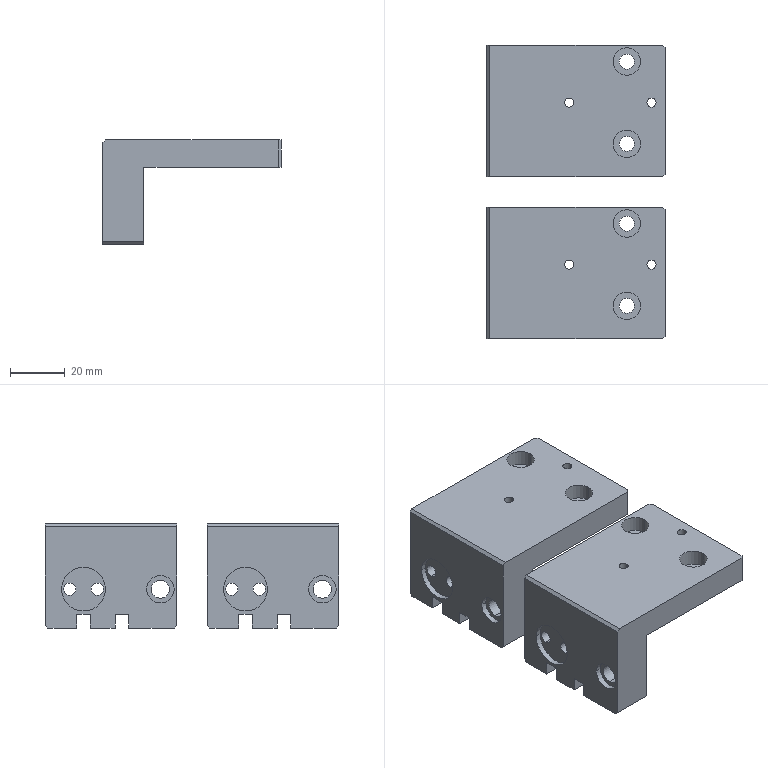NC program | NX | posted with a generic post | part box 65 x 107 x 38 mm
Lines 65 to 929 of 5955:
(ZLEVEL_PROFILE , TOOL : D10)
N110 T15 M6
N112 G54
N114 G17 G0 G90 X45.832 Y37.6 B0. C0. S9500 M3
N116 G43 Z30. H15
N118 Z1.5
N120 G94 G1 X54.054 Z1.069 F1000.
N122 X55.398 Y37.266 Z0.996
N124 X56.604 Y36.584 Z0.924
N126 X57.584 Y35.604 Z0.851
N128 X58.266 Y34.398 Z0.779
N130 X58.6 Y33.054 Z0.706
N132 Y0.5 Z-1.
N134 Y-31.5 F3000.
N136 G2 X57.106 Y-35.106 R5.1
N138 G1 X56.106 Y-36.106
N140 G2 X52.5 Y-37.6 R5.1
N142 G1 X6.5
N144 G2 X2.894 Y-36.106 R5.1
N146 G1 X1.894 Y-35.106
N148 G2 X0.4 Y-31.5 R5.1
N150 G1 Y32.5
N152 G2 X5.5 Y37.6 R5.1
N154 G1 X53.5
N156 G2 X58.6 Y32.5 R5.1
N158 G1 Y0.5
N160 Y-31.5 Z-1.125
N162 X58.575 Y-32. Z-1.127
N164 X58.502 Y-32.495 Z-1.128
N166 X58.38 Y-32.98 Z-1.13
N168 X58.212 Y-33.452 Z-1.132
N170 X57.998 Y-33.904 Z-1.134
N172 X57.74 Y-34.333 Z-1.136
N174 X57.442 Y-34.735 Z-1.138
N176 X57.106 Y-35.106 Z-1.14
N178 X56.106 Y-36.106 Z-1.146
N180 X55.735 Y-36.442 Z-1.148
N182 X55.333 Y-36.74 Z-1.15
N184 X54.904 Y-36.998 Z-1.152
N186 X54.452 Y-37.212 Z-1.153
N188 X53.98 Y-37.38 Z-1.155
N190 X53.495 Y-37.502 Z-1.157
N192 X53. Y-37.575 Z-1.159
N194 X52.5 Y-37.6 Z-1.161
N196 X6.5 Z-1.34
N198 X6. Y-37.575 Z-1.342
N200 X5.505 Y-37.502 Z-1.344
N202 X5.02 Y-37.38 Z-1.346
N204 X4.548 Y-37.212 Z-1.348
N206 X4.096 Y-36.998 Z-1.35
N208 X3.667 Y-36.74 Z-1.352
N210 X3.265 Y-36.442 Z-1.354
N212 X2.894 Y-36.106 Z-1.356
N214 X1.894 Y-35.106 Z-1.361
N216 X1.558 Y-34.735 Z-1.363
N218 X1.26 Y-34.333 Z-1.365
N220 X1.002 Y-33.904 Z-1.367
N222 X0.788 Y-33.452 Z-1.369
N224 X0.62 Y-32.98 Z-1.371
N226 X0.498 Y-32.495 Z-1.373
N228 X0.425 Y-32. Z-1.375
N230 X0.4 Y-31.5 Z-1.377
N232 Y32.5 Z-1.626
N234 X0.425 Y33. Z-1.628
N236 X0.498 Y33.495 Z-1.63
N238 X0.62 Y33.98 Z-1.632
N240 X0.788 Y34.452 Z-1.634
N242 X1.002 Y34.904 Z-1.636
N244 X1.26 Y35.333 Z-1.638
N246 X1.558 Y35.735 Z-1.64
N248 X1.894 Y36.106 Z-1.642
N250 X2.265 Y36.442 Z-1.644
N252 X2.667 Y36.74 Z-1.646
N254 X3.096 Y36.998 Z-1.648
N256 X3.548 Y37.212 Z-1.65
N258 X4.02 Y37.38 Z-1.652
N260 X4.505 Y37.502 Z-1.653
N262 X5. Y37.575 Z-1.655
N264 X5.5 Y37.6 Z-1.657
N266 X53.5 Z-1.844
N268 X54. Y37.575 Z-1.846
N270 X54.495 Y37.502 Z-1.848
N272 X54.98 Y37.38 Z-1.85
N274 X55.452 Y37.212 Z-1.852
N276 X55.904 Y36.998 Z-1.854
N278 X56.333 Y36.74 Z-1.856
N280 X56.735 Y36.442 Z-1.858
N282 X57.106 Y36.106 Z-1.86
N284 X57.442 Y35.735 Z-1.862
N286 X57.74 Y35.333 Z-1.864
N288 X57.998 Y34.904 Z-1.866
N290 X58.212 Y34.452 Z-1.868
N292 X58.38 Y33.98 Z-1.87
N294 X58.502 Y33.495 Z-1.872
N296 X58.575 Y33. Z-1.873
N298 X58.6 Y32.5 Z-1.875
N300 Y0.5 Z-2.
N302 Y-31.5 Z-2.125
N304 X58.575 Y-32. Z-2.127
N306 X58.502 Y-32.495 Z-2.128
N308 X58.38 Y-32.98 Z-2.13
N310 X58.212 Y-33.452 Z-2.132
N312 X57.998 Y-33.904 Z-2.134
N314 X57.74 Y-34.333 Z-2.136
N316 X57.442 Y-34.735 Z-2.138
N318 X57.106 Y-35.106 Z-2.14
N320 X56.106 Y-36.106 Z-2.146
N322 X55.735 Y-36.442 Z-2.148
N324 X55.333 Y-36.74 Z-2.15
N326 X54.904 Y-36.998 Z-2.152
N328 X54.452 Y-37.212 Z-2.153
N330 X53.98 Y-37.38 Z-2.155
N332 X53.495 Y-37.502 Z-2.157
N334 X53. Y-37.575 Z-2.159
N336 X52.5 Y-37.6 Z-2.161
N338 X6.5 Z-2.34
N340 X6. Y-37.575 Z-2.342
N342 X5.505 Y-37.502 Z-2.344
N344 X5.02 Y-37.38 Z-2.346
N346 X4.548 Y-37.212 Z-2.348
N348 X4.096 Y-36.998 Z-2.35
N350 X3.667 Y-36.74 Z-2.352
N352 X3.265 Y-36.442 Z-2.354
N354 X2.894 Y-36.106 Z-2.356
N356 X1.894 Y-35.106 Z-2.361
N358 X1.558 Y-34.735 Z-2.363
N360 X1.26 Y-34.333 Z-2.365
N362 X1.002 Y-33.904 Z-2.367
N364 X0.788 Y-33.452 Z-2.369
N366 X0.62 Y-32.98 Z-2.371
N368 X0.498 Y-32.495 Z-2.373
N370 X0.425 Y-32. Z-2.375
N372 X0.4 Y-31.5 Z-2.377
N374 Y32.5 Z-2.626
N376 X0.425 Y33. Z-2.628
N378 X0.498 Y33.495 Z-2.63
N380 X0.62 Y33.98 Z-2.632
N382 X0.788 Y34.452 Z-2.634
N384 X1.002 Y34.904 Z-2.636
N386 X1.26 Y35.333 Z-2.638
N388 X1.558 Y35.735 Z-2.64
N390 X1.894 Y36.106 Z-2.642
N392 X2.265 Y36.442 Z-2.644
N394 X2.667 Y36.74 Z-2.646
N396 X3.096 Y36.998 Z-2.648
N398 X3.548 Y37.212 Z-2.65
N400 X4.02 Y37.38 Z-2.652
N402 X4.505 Y37.502 Z-2.653
N404 X5. Y37.575 Z-2.655
N406 X5.5 Y37.6 Z-2.657
N408 X53.5 Z-2.844
N410 X54. Y37.575 Z-2.846
N412 X54.495 Y37.502 Z-2.848
N414 X54.98 Y37.38 Z-2.85
N416 X55.452 Y37.212 Z-2.852
N418 X55.904 Y36.998 Z-2.854
N420 X56.333 Y36.74 Z-2.856
N422 X56.735 Y36.442 Z-2.858
N424 X57.106 Y36.106 Z-2.86
N426 X57.442 Y35.735 Z-2.862
N428 X57.74 Y35.333 Z-2.864
N430 X57.998 Y34.904 Z-2.866
N432 X58.212 Y34.452 Z-2.868
N434 X58.38 Y33.98 Z-2.87
N436 X58.502 Y33.495 Z-2.872
N438 X58.575 Y33. Z-2.873
N440 X58.6 Y32.5 Z-2.875
N442 Y0.5 Z-3.
N444 Y-31.5 Z-3.125
N446 X58.575 Y-32. Z-3.127
N448 X58.502 Y-32.495 Z-3.128
N450 X58.38 Y-32.98 Z-3.13
N452 X58.212 Y-33.452 Z-3.132
N454 X57.998 Y-33.904 Z-3.134
N456 X57.74 Y-34.333 Z-3.136
N458 X57.442 Y-34.735 Z-3.138
N460 X57.106 Y-35.106 Z-3.14
N462 X56.106 Y-36.106 Z-3.146
N464 X55.735 Y-36.442 Z-3.148
N466 X55.333 Y-36.74 Z-3.15
N468 X54.904 Y-36.998 Z-3.152
N470 X54.452 Y-37.212 Z-3.153
N472 X53.98 Y-37.38 Z-3.155
N474 X53.495 Y-37.502 Z-3.157
N476 X53. Y-37.575 Z-3.159
N478 X52.5 Y-37.6 Z-3.161
N480 X6.5 Z-3.34
N482 X6. Y-37.575 Z-3.342
N484 X5.505 Y-37.502 Z-3.344
N486 X5.02 Y-37.38 Z-3.346
N488 X4.548 Y-37.212 Z-3.348
N490 X4.096 Y-36.998 Z-3.35
N492 X3.667 Y-36.74 Z-3.352
N494 X3.265 Y-36.442 Z-3.354
N496 X2.894 Y-36.106 Z-3.356
N498 X1.894 Y-35.106 Z-3.361
N500 X1.558 Y-34.735 Z-3.363
N502 X1.26 Y-34.333 Z-3.365
N504 X1.002 Y-33.904 Z-3.367
N506 X0.788 Y-33.452 Z-3.369
N508 X0.62 Y-32.98 Z-3.371
N510 X0.498 Y-32.495 Z-3.373
N512 X0.425 Y-32. Z-3.375
N514 X0.4 Y-31.5 Z-3.377
N516 Y32.5 Z-3.626
N518 X0.425 Y33. Z-3.628
N520 X0.498 Y33.495 Z-3.63
N522 X0.62 Y33.98 Z-3.632
N524 X0.788 Y34.452 Z-3.634
N526 X1.002 Y34.904 Z-3.636
N528 X1.26 Y35.333 Z-3.638
N530 X1.558 Y35.735 Z-3.64
N532 X1.894 Y36.106 Z-3.642
N534 X2.265 Y36.442 Z-3.644
N536 X2.667 Y36.74 Z-3.646
N538 X3.096 Y36.998 Z-3.648
N540 X3.548 Y37.212 Z-3.65
N542 X4.02 Y37.38 Z-3.652
N544 X4.505 Y37.502 Z-3.653
N546 X5. Y37.575 Z-3.655
N548 X5.5 Y37.6 Z-3.657
N550 X53.5 Z-3.844
N552 X54. Y37.575 Z-3.846
N554 X54.495 Y37.502 Z-3.848
N556 X54.98 Y37.38 Z-3.85
N558 X55.452 Y37.212 Z-3.852
N560 X55.904 Y36.998 Z-3.854
N562 X56.333 Y36.74 Z-3.856
N564 X56.735 Y36.442 Z-3.858
N566 X57.106 Y36.106 Z-3.86
N568 X57.442 Y35.735 Z-3.862
N570 X57.74 Y35.333 Z-3.864
N572 X57.998 Y34.904 Z-3.866
N574 X58.212 Y34.452 Z-3.868
N576 X58.38 Y33.98 Z-3.87
N578 X58.502 Y33.495 Z-3.872
N580 X58.575 Y33. Z-3.873
N582 X58.6 Y32.5 Z-3.875
N584 Y0.5 Z-4.
N586 Y-31.5 Z-4.125
N588 X58.575 Y-32. Z-4.127
N590 X58.502 Y-32.495 Z-4.128
N592 X58.38 Y-32.98 Z-4.13
N594 X58.212 Y-33.452 Z-4.132
N596 X57.998 Y-33.904 Z-4.134
N598 X57.74 Y-34.333 Z-4.136
N600 X57.442 Y-34.735 Z-4.138
N602 X57.106 Y-35.106 Z-4.14
N604 X56.106 Y-36.106 Z-4.146
N606 X55.735 Y-36.442 Z-4.148
N608 X55.333 Y-36.74 Z-4.15
N610 X54.904 Y-36.998 Z-4.152
N612 X54.452 Y-37.212 Z-4.153
N614 X53.98 Y-37.38 Z-4.155
N616 X53.495 Y-37.502 Z-4.157
N618 X53. Y-37.575 Z-4.159
N620 X52.5 Y-37.6 Z-4.161
N622 X6.5 Z-4.34
N624 X6. Y-37.575 Z-4.342
N626 X5.505 Y-37.502 Z-4.344
N628 X5.02 Y-37.38 Z-4.346
N630 X4.548 Y-37.212 Z-4.348
N632 X4.096 Y-36.998 Z-4.35
N634 X3.667 Y-36.74 Z-4.352
N636 X3.265 Y-36.442 Z-4.354
N638 X2.894 Y-36.106 Z-4.356
N640 X1.894 Y-35.106 Z-4.361
N642 X1.558 Y-34.735 Z-4.363
N644 X1.26 Y-34.333 Z-4.365
N646 X1.002 Y-33.904 Z-4.367
N648 X0.788 Y-33.452 Z-4.369
N650 X0.62 Y-32.98 Z-4.371
N652 X0.498 Y-32.495 Z-4.373
N654 X0.425 Y-32. Z-4.375
N656 X0.4 Y-31.5 Z-4.377
N658 Y32.5 Z-4.626
N660 X0.425 Y33. Z-4.628
N662 X0.498 Y33.495 Z-4.63
N664 X0.62 Y33.98 Z-4.632
N666 X0.788 Y34.452 Z-4.634
N668 X1.002 Y34.904 Z-4.636
N670 X1.26 Y35.333 Z-4.638
N672 X1.558 Y35.735 Z-4.64
N674 X1.894 Y36.106 Z-4.642
N676 X2.265 Y36.442 Z-4.644
N678 X2.667 Y36.74 Z-4.646
N680 X3.096 Y36.998 Z-4.648
N682 X3.548 Y37.212 Z-4.65
N684 X4.02 Y37.38 Z-4.652
N686 X4.505 Y37.502 Z-4.653
N688 X5. Y37.575 Z-4.655
N690 X5.5 Y37.6 Z-4.657
N692 X53.5 Z-4.844
N694 X54. Y37.575 Z-4.846
N696 X54.495 Y37.502 Z-4.848
N698 X54.98 Y37.38 Z-4.85
N700 X55.452 Y37.212 Z-4.852
N702 X55.904 Y36.998 Z-4.854
N704 X56.333 Y36.74 Z-4.856
N706 X56.735 Y36.442 Z-4.858
N708 X57.106 Y36.106 Z-4.86
N710 X57.442 Y35.735 Z-4.862
N712 X57.74 Y35.333 Z-4.864
N714 X57.998 Y34.904 Z-4.866
N716 X58.212 Y34.452 Z-4.868
N718 X58.38 Y33.98 Z-4.87
N720 X58.502 Y33.495 Z-4.872
N722 X58.575 Y33. Z-4.873
N724 X58.6 Y32.5 Z-4.875
N726 Y0.5 Z-5.
N728 Y-31.5 Z-5.125
N730 X58.575 Y-32. Z-5.127
N732 X58.502 Y-32.495 Z-5.128
N734 X58.38 Y-32.98 Z-5.13
N736 X58.212 Y-33.452 Z-5.132
N738 X57.998 Y-33.904 Z-5.134
N740 X57.74 Y-34.333 Z-5.136
N742 X57.442 Y-34.735 Z-5.138
N744 X57.106 Y-35.106 Z-5.14
N746 X56.106 Y-36.106 Z-5.146
N748 X55.735 Y-36.442 Z-5.148
N750 X55.333 Y-36.74 Z-5.15
N752 X54.904 Y-36.998 Z-5.152
N754 X54.452 Y-37.212 Z-5.153
N756 X53.98 Y-37.38 Z-5.155
N758 X53.495 Y-37.502 Z-5.157
N760 X53. Y-37.575 Z-5.159
N762 X52.5 Y-37.6 Z-5.161
N764 X6.5 Z-5.34
N766 X6. Y-37.575 Z-5.342
N768 X5.505 Y-37.502 Z-5.344
N770 X5.02 Y-37.38 Z-5.346
N772 X4.548 Y-37.212 Z-5.348
N774 X4.096 Y-36.998 Z-5.35
N776 X3.667 Y-36.74 Z-5.352
N778 X3.265 Y-36.442 Z-5.354
N780 X2.894 Y-36.106 Z-5.356
N782 X1.894 Y-35.106 Z-5.361
N784 X1.558 Y-34.735 Z-5.363
N786 X1.26 Y-34.333 Z-5.365
N788 X1.002 Y-33.904 Z-5.367
N790 X0.788 Y-33.452 Z-5.369
N792 X0.62 Y-32.98 Z-5.371
N794 X0.498 Y-32.495 Z-5.373
N796 X0.425 Y-32. Z-5.375
N798 X0.4 Y-31.5 Z-5.377
N800 Y32.5 Z-5.626
N802 X0.425 Y33. Z-5.628
N804 X0.498 Y33.495 Z-5.63
N806 X0.62 Y33.98 Z-5.632
N808 X0.788 Y34.452 Z-5.634
N810 X1.002 Y34.904 Z-5.636
N812 X1.26 Y35.333 Z-5.638
N814 X1.558 Y35.735 Z-5.64
N816 X1.894 Y36.106 Z-5.642
N818 X2.265 Y36.442 Z-5.644
N820 X2.667 Y36.74 Z-5.646
N822 X3.096 Y36.998 Z-5.648
N824 X3.548 Y37.212 Z-5.65
N826 X4.02 Y37.38 Z-5.652
N828 X4.505 Y37.502 Z-5.653
N830 X5. Y37.575 Z-5.655
N832 X5.5 Y37.6 Z-5.657
N834 X53.5 Z-5.844
N836 X54. Y37.575 Z-5.846
N838 X54.495 Y37.502 Z-5.848
N840 X54.98 Y37.38 Z-5.85
N842 X55.452 Y37.212 Z-5.852
N844 X55.904 Y36.998 Z-5.854
N846 X56.333 Y36.74 Z-5.856
N848 X56.735 Y36.442 Z-5.858
N850 X57.106 Y36.106 Z-5.86
N852 X57.442 Y35.735 Z-5.862
N854 X57.74 Y35.333 Z-5.864
N856 X57.998 Y34.904 Z-5.866
N858 X58.212 Y34.452 Z-5.868
N860 X58.38 Y33.98 Z-5.87
N862 X58.502 Y33.495 Z-5.872
N864 X58.575 Y33. Z-5.873
N866 X58.6 Y32.5 Z-5.875
N868 Y0.5 Z-6.
N870 Y-31.5 Z-6.125
N872 X58.575 Y-32. Z-6.127
N874 X58.502 Y-32.495 Z-6.128
N876 X58.38 Y-32.98 Z-6.13
N878 X58.212 Y-33.452 Z-6.132
N880 X57.998 Y-33.904 Z-6.134
N882 X57.74 Y-34.333 Z-6.136
N884 X57.442 Y-34.735 Z-6.138
N886 X57.106 Y-35.106 Z-6.14
N888 X56.106 Y-36.106 Z-6.146
N890 X55.735 Y-36.442 Z-6.148
N892 X55.333 Y-36.74 Z-6.15
N894 X54.904 Y-36.998 Z-6.152
N896 X54.452 Y-37.212 Z-6.153
N898 X53.98 Y-37.38 Z-6.155
N900 X53.495 Y-37.502 Z-6.157
N902 X53. Y-37.575 Z-6.159
N904 X52.5 Y-37.6 Z-6.161
N906 X6.5 Z-6.34
N908 X6. Y-37.575 Z-6.342
N910 X5.505 Y-37.502 Z-6.344
N912 X5.02 Y-37.38 Z-6.346
N914 X4.548 Y-37.212 Z-6.348
N916 X4.096 Y-36.998 Z-6.35
N918 X3.667 Y-36.74 Z-6.352
N920 X3.265 Y-36.442 Z-6.354
N922 X2.894 Y-36.106 Z-6.356
N924 X1.894 Y-35.106 Z-6.361
N926 X1.558 Y-34.735 Z-6.363
N928 X1.26 Y-34.333 Z-6.365
N930 X1.002 Y-33.904 Z-6.367
N932 X0.788 Y-33.452 Z-6.369
N934 X0.62 Y-32.98 Z-6.371
N936 X0.498 Y-32.495 Z-6.373
N938 X0.425 Y-32. Z-6.375
N940 X0.4 Y-31.5 Z-6.377
N942 Y32.5 Z-6.626
N944 X0.425 Y33. Z-6.628
N946 X0.498 Y33.495 Z-6.63
N948 X0.62 Y33.98 Z-6.632
N950 X0.788 Y34.452 Z-6.634
N952 X1.002 Y34.904 Z-6.636
N954 X1.26 Y35.333 Z-6.638
N956 X1.558 Y35.735 Z-6.64
N958 X1.894 Y36.106 Z-6.642
N960 X2.265 Y36.442 Z-6.644
N962 X2.667 Y36.74 Z-6.646
N964 X3.096 Y36.998 Z-6.648
N966 X3.548 Y37.212 Z-6.65
N968 X4.02 Y37.38 Z-6.652
N970 X4.505 Y37.502 Z-6.653
N972 X5. Y37.575 Z-6.655
N974 X5.5 Y37.6 Z-6.657
N976 X53.5 Z-6.844
N978 X54. Y37.575 Z-6.846
N980 X54.495 Y37.502 Z-6.848
N982 X54.98 Y37.38 Z-6.85
N984 X55.452 Y37.212 Z-6.852
N986 X55.904 Y36.998 Z-6.854
N988 X56.333 Y36.74 Z-6.856
N990 X56.735 Y36.442 Z-6.858
N992 X57.106 Y36.106 Z-6.86
N994 X57.442 Y35.735 Z-6.862
N996 X57.74 Y35.333 Z-6.864
N998 X57.998 Y34.904 Z-6.866
N1000 X58.212 Y34.452 Z-6.868
N1002 X58.38 Y33.98 Z-6.87
N1004 X58.502 Y33.495 Z-6.872
N1006 X58.575 Y33. Z-6.873
N1008 X58.6 Y32.5 Z-6.875
N1010 Y0.5 Z-7.
N1012 Y-31.5 Z-7.125
N1014 X58.575 Y-32. Z-7.127
N1016 X58.502 Y-32.495 Z-7.128
N1018 X58.38 Y-32.98 Z-7.13
N1020 X58.212 Y-33.452 Z-7.132
N1022 X57.998 Y-33.904 Z-7.134
N1024 X57.74 Y-34.333 Z-7.136
N1026 X57.442 Y-34.735 Z-7.138
N1028 X57.106 Y-35.106 Z-7.14
N1030 X56.106 Y-36.106 Z-7.146
N1032 X55.735 Y-36.442 Z-7.148
N1034 X55.333 Y-36.74 Z-7.15
N1036 X54.904 Y-36.998 Z-7.152
N1038 X54.452 Y-37.212 Z-7.153
N1040 X53.98 Y-37.38 Z-7.155
N1042 X53.495 Y-37.502 Z-7.157
N1044 X53. Y-37.575 Z-7.159
N1046 X52.5 Y-37.6 Z-7.161
N1048 X6.5 Z-7.34
N1050 X6. Y-37.575 Z-7.342
N1052 X5.505 Y-37.502 Z-7.344
N1054 X5.02 Y-37.38 Z-7.346
N1056 X4.548 Y-37.212 Z-7.348
N1058 X4.096 Y-36.998 Z-7.35
N1060 X3.667 Y-36.74 Z-7.352
N1062 X3.265 Y-36.442 Z-7.354
N1064 X2.894 Y-36.106 Z-7.356
N1066 X1.894 Y-35.106 Z-7.361
N1068 X1.558 Y-34.735 Z-7.363
N1070 X1.26 Y-34.333 Z-7.365
N1072 X1.002 Y-33.904 Z-7.367
N1074 X0.788 Y-33.452 Z-7.369
N1076 X0.62 Y-32.98 Z-7.371
N1078 X0.498 Y-32.495 Z-7.373
N1080 X0.425 Y-32. Z-7.375
N1082 X0.4 Y-31.5 Z-7.377
N1084 Y32.5 Z-7.626
N1086 X0.425 Y33. Z-7.628
N1088 X0.498 Y33.495 Z-7.63
N1090 X0.62 Y33.98 Z-7.632
N1092 X0.788 Y34.452 Z-7.634
N1094 X1.002 Y34.904 Z-7.636
N1096 X1.26 Y35.333 Z-7.638
N1098 X1.558 Y35.735 Z-7.64
N1100 X1.894 Y36.106 Z-7.642
N1102 X2.265 Y36.442 Z-7.644
N1104 X2.667 Y36.74 Z-7.646
N1106 X3.096 Y36.998 Z-7.648
N1108 X3.548 Y37.212 Z-7.65
N1110 X4.02 Y37.38 Z-7.652
N1112 X4.505 Y37.502 Z-7.653
N1114 X5. Y37.575 Z-7.655
N1116 X5.5 Y37.6 Z-7.657
N1118 X53.5 Z-7.844
N1120 X54. Y37.575 Z-7.846
N1122 X54.495 Y37.502 Z-7.848
N1124 X54.98 Y37.38 Z-7.85
N1126 X55.452 Y37.212 Z-7.852
N1128 X55.904 Y36.998 Z-7.854
N1130 X56.333 Y36.74 Z-7.856
N1132 X56.735 Y36.442 Z-7.858
N1134 X57.106 Y36.106 Z-7.86
N1136 X57.442 Y35.735 Z-7.862
N1138 X57.74 Y35.333 Z-7.864
N1140 X57.998 Y34.904 Z-7.866
N1142 X58.212 Y34.452 Z-7.868
N1144 X58.38 Y33.98 Z-7.87
N1146 X58.502 Y33.495 Z-7.872
N1148 X58.575 Y33. Z-7.873
N1150 X58.6 Y32.5 Z-7.875
N1152 Y0.5 Z-8.
N1154 Y-31.5 Z-8.125
N1156 X58.575 Y-32. Z-8.127
N1158 X58.502 Y-32.495 Z-8.128
N1160 X58.38 Y-32.98 Z-8.13
N1162 X58.212 Y-33.452 Z-8.132
N1164 X57.998 Y-33.904 Z-8.134
N1166 X57.74 Y-34.333 Z-8.136
N1168 X57.442 Y-34.735 Z-8.138
N1170 X57.106 Y-35.106 Z-8.14
N1172 X56.106 Y-36.106 Z-8.146
N1174 X55.735 Y-36.442 Z-8.148
N1176 X55.333 Y-36.74 Z-8.15
N1178 X54.904 Y-36.998 Z-8.152
N1180 X54.452 Y-37.212 Z-8.153
N1182 X53.98 Y-37.38 Z-8.155
N1184 X53.495 Y-37.502 Z-8.157
N1186 X53. Y-37.575 Z-8.159
N1188 X52.5 Y-37.6 Z-8.161
N1190 X6.5 Z-8.34
N1192 X6. Y-37.575 Z-8.342
N1194 X5.505 Y-37.502 Z-8.344
N1196 X5.02 Y-37.38 Z-8.346
N1198 X4.548 Y-37.212 Z-8.348
N1200 X4.096 Y-36.998 Z-8.35
N1202 X3.667 Y-36.74 Z-8.352
N1204 X3.265 Y-36.442 Z-8.354
N1206 X2.894 Y-36.106 Z-8.356
N1208 X1.894 Y-35.106 Z-8.361
N1210 X1.558 Y-34.735 Z-8.363
N1212 X1.26 Y-34.333 Z-8.365
N1214 X1.002 Y-33.904 Z-8.367
N1216 X0.788 Y-33.452 Z-8.369
N1218 X0.62 Y-32.98 Z-8.371
N1220 X0.498 Y-32.495 Z-8.373
N1222 X0.425 Y-32. Z-8.375
N1224 X0.4 Y-31.5 Z-8.377
N1226 Y32.5 Z-8.626
N1228 X0.425 Y33. Z-8.628
N1230 X0.498 Y33.495 Z-8.63
N1232 X0.62 Y33.98 Z-8.632
N1234 X0.788 Y34.452 Z-8.634
N1236 X1.002 Y34.904 Z-8.636
N1238 X1.26 Y35.333 Z-8.638
N1240 X1.558 Y35.735 Z-8.64
N1242 X1.894 Y36.106 Z-8.642
N1244 X2.265 Y36.442 Z-8.644
N1246 X2.667 Y36.74 Z-8.646
N1248 X3.096 Y36.998 Z-8.648
N1250 X3.548 Y37.212 Z-8.65
N1252 X4.02 Y37.38 Z-8.652
N1254 X4.505 Y37.502 Z-8.653
N1256 X5. Y37.575 Z-8.655
N1258 X5.5 Y37.6 Z-8.657
N1260 X53.5 Z-8.844
N1262 X54. Y37.575 Z-8.846
N1264 X54.495 Y37.502 Z-8.848
N1266 X54.98 Y37.38 Z-8.85
N1268 X55.452 Y37.212 Z-8.852
N1270 X55.904 Y36.998 Z-8.854
N1272 X56.333 Y36.74 Z-8.856
N1274 X56.735 Y36.442 Z-8.858
N1276 X57.106 Y36.106 Z-8.86
N1278 X57.442 Y35.735 Z-8.862
N1280 X57.74 Y35.333 Z-8.864
N1282 X57.998 Y34.904 Z-8.866
N1284 X58.212 Y34.452 Z-8.868
N1286 X58.38 Y33.98 Z-8.87
N1288 X58.502 Y33.495 Z-8.872
N1290 X58.575 Y33. Z-8.873
N1292 X58.6 Y32.5 Z-8.875
N1294 Y0.5 Z-9.
N1296 Y-31.5 Z-9.125
N1298 X58.575 Y-32. Z-9.127
N1300 X58.502 Y-32.495 Z-9.128
N1302 X58.38 Y-32.98 Z-9.13
N1304 X58.212 Y-33.452 Z-9.132
N1306 X57.998 Y-33.904 Z-9.134
N1308 X57.74 Y-34.333 Z-9.136
N1310 X57.442 Y-34.735 Z-9.138
N1312 X57.106 Y-35.106 Z-9.14
N1314 X56.106 Y-36.106 Z-9.146
N1316 X55.735 Y-36.442 Z-9.148
N1318 X55.333 Y-36.74 Z-9.15
N1320 X54.904 Y-36.998 Z-9.152
N1322 X54.452 Y-37.212 Z-9.153
N1324 X53.98 Y-37.38 Z-9.155
N1326 X53.495 Y-37.502 Z-9.157
N1328 X53. Y-37.575 Z-9.159
N1330 X52.5 Y-37.6 Z-9.161
N1332 X6.5 Z-9.34
N1334 X6. Y-37.575 Z-9.342
N1336 X5.505 Y-37.502 Z-9.344
N1338 X5.02 Y-37.38 Z-9.346
N1340 X4.548 Y-37.212 Z-9.348
N1342 X4.096 Y-36.998 Z-9.35
N1344 X3.667 Y-36.74 Z-9.352
N1346 X3.265 Y-36.442 Z-9.354
N1348 X2.894 Y-36.106 Z-9.356
N1350 X1.894 Y-35.106 Z-9.361
N1352 X1.558 Y-34.735 Z-9.363
N1354 X1.26 Y-34.333 Z-9.365
N1356 X1.002 Y-33.904 Z-9.367
N1358 X0.788 Y-33.452 Z-9.369
N1360 X0.62 Y-32.98 Z-9.371
N1362 X0.498 Y-32.495 Z-9.373
N1364 X0.425 Y-32. Z-9.375
N1366 X0.4 Y-31.5 Z-9.377
N1368 Y32.5 Z-9.626
N1370 X0.425 Y33. Z-9.628
N1372 X0.498 Y33.495 Z-9.63
N1374 X0.62 Y33.98 Z-9.632
N1376 X0.788 Y34.452 Z-9.634
N1378 X1.002 Y34.904 Z-9.636
N1380 X1.26 Y35.333 Z-9.638
N1382 X1.558 Y35.735 Z-9.64
N1384 X1.894 Y36.106 Z-9.642
N1386 X2.265 Y36.442 Z-9.644
N1388 X2.667 Y36.74 Z-9.646
N1390 X3.096 Y36.998 Z-9.648
N1392 X3.548 Y37.212 Z-9.65
N1394 X4.02 Y37.38 Z-9.652
N1396 X4.505 Y37.502 Z-9.653
N1398 X5. Y37.575 Z-9.655
N1400 X5.5 Y37.6 Z-9.657
N1402 X53.5 Z-9.844
N1404 X54. Y37.575 Z-9.846
N1406 X54.495 Y37.502 Z-9.848
N1408 X54.98 Y37.38 Z-9.85
N1410 X55.452 Y37.212 Z-9.852
N1412 X55.904 Y36.998 Z-9.854
N1414 X56.333 Y36.74 Z-9.856
N1416 X56.735 Y36.442 Z-9.858
N1418 X57.106 Y36.106 Z-9.86
N1420 X57.442 Y35.735 Z-9.862
N1422 X57.74 Y35.333 Z-9.864
N1424 X57.998 Y34.904 Z-9.866
N1426 X58.212 Y34.452 Z-9.868
N1428 X58.38 Y33.98 Z-9.87
N1430 X58.502 Y33.495 Z-9.872
N1432 X58.575 Y33. Z-9.873
N1434 X58.6 Y32.5 Z-9.875
N1436 Y0.5 Z-10.
N1438 Y-31.5 Z-10.125
N1440 X58.575 Y-32. Z-10.127
N1442 X58.502 Y-32.495 Z-10.128
N1444 X58.38 Y-32.98 Z-10.13
N1446 X58.212 Y-33.452 Z-10.132
N1448 X57.998 Y-33.904 Z-10.134
N1450 X57.74 Y-34.333 Z-10.136
N1452 X57.442 Y-34.735 Z-10.138
N1454 X57.106 Y-35.106 Z-10.14
N1456 X56.106 Y-36.106 Z-10.146
N1458 X55.735 Y-36.442 Z-10.148
N1460 X55.333 Y-36.74 Z-10.15
N1462 X54.904 Y-36.998 Z-10.152
N1464 X54.452 Y-37.212 Z-10.153
N1466 X53.98 Y-37.38 Z-10.155
N1468 X53.495 Y-37.502 Z-10.157
N1470 X53. Y-37.575 Z-10.159
N1472 X52.5 Y-37.6 Z-10.161
N1474 X6.5 Z-10.34
N1476 X6. Y-37.575 Z-10.342
N1478 X5.505 Y-37.502 Z-10.344
N1480 X5.02 Y-37.38 Z-10.346
N1482 X4.548 Y-37.212 Z-10.348
N1484 X4.096 Y-36.998 Z-10.35
N1486 X3.667 Y-36.74 Z-10.352
N1488 X3.265 Y-36.442 Z-10.354
N1490 X2.894 Y-36.106 Z-10.356
N1492 X1.894 Y-35.106 Z-10.361
N1494 X1.558 Y-34.735 Z-10.363
N1496 X1.26 Y-34.333 Z-10.365
N1498 X1.002 Y-33.904 Z-10.367
N1500 X0.788 Y-33.452 Z-10.369
N1502 X0.62 Y-32.98 Z-10.371
N1504 X0.498 Y-32.495 Z-10.373
N1506 X0.425 Y-32. Z-10.375
N1508 X0.4 Y-31.5 Z-10.377
N1510 Y32.5 Z-10.626
N1512 X0.425 Y33. Z-10.628
N1514 X0.498 Y33.495 Z-10.63
N1516 X0.62 Y33.98 Z-10.632
N1518 X0.788 Y34.452 Z-10.634
N1520 X1.002 Y34.904 Z-10.636
N1522 X1.26 Y35.333 Z-10.638
N1524 X1.558 Y35.735 Z-10.64
N1526 X1.894 Y36.106 Z-10.642
N1528 X2.265 Y36.442 Z-10.644
N1530 X2.667 Y36.74 Z-10.646
N1532 X3.096 Y36.998 Z-10.648
N1534 X3.548 Y37.212 Z-10.65
N1536 X4.02 Y37.38 Z-10.652
N1538 X4.505 Y37.502 Z-10.653
N1540 X5. Y37.575 Z-10.655
N1542 X5.5 Y37.6 Z-10.657
N1544 X53.5 Z-10.844
N1546 X54. Y37.575 Z-10.846
N1548 X54.495 Y37.502 Z-10.848
N1550 X54.98 Y37.38 Z-10.85
N1552 X55.452 Y37.212 Z-10.852
N1554 X55.904 Y36.998 Z-10.854
N1556 X56.333 Y36.74 Z-10.856
N1558 X56.735 Y36.442 Z-10.858
N1560 X57.106 Y36.106 Z-10.86
N1562 X57.442 Y35.735 Z-10.862
N1564 X57.74 Y35.333 Z-10.864
N1566 X57.998 Y34.904 Z-10.866
N1568 X58.212 Y34.452 Z-10.868
N1570 X58.38 Y33.98 Z-10.87
N1572 X58.502 Y33.495 Z-10.872
N1574 X58.575 Y33. Z-10.873
N1576 X58.6 Y32.5 Z-10.875
N1578 Y0.5 Z-11.
N1580 Y-31.5 Z-11.125
N1582 X58.575 Y-32. Z-11.127
N1584 X58.502 Y-32.495 Z-11.128
N1586 X58.38 Y-32.98 Z-11.13
N1588 X58.212 Y-33.452 Z-11.132
N1590 X57.998 Y-33.904 Z-11.134
N1592 X57.74 Y-34.333 Z-11.136
N1594 X57.442 Y-34.735 Z-11.138
N1596 X57.106 Y-35.106 Z-11.14
N1598 X56.106 Y-36.106 Z-11.146
N1600 X55.735 Y-36.442 Z-11.148
N1602 X55.333 Y-36.74 Z-11.15
N1604 X54.904 Y-36.998 Z-11.152
N1606 X54.452 Y-37.212 Z-11.153
N1608 X53.98 Y-37.38 Z-11.155
N1610 X53.495 Y-37.502 Z-11.157
N1612 X53. Y-37.575 Z-11.159
N1614 X52.5 Y-37.6 Z-11.161
N1616 X6.5 Z-11.34
N1618 X6. Y-37.575 Z-11.342
N1620 X5.505 Y-37.502 Z-11.344
N1622 X5.02 Y-37.38 Z-11.346
N1624 X4.548 Y-37.212 Z-11.348
N1626 X4.096 Y-36.998 Z-11.35
N1628 X3.667 Y-36.74 Z-11.352
N1630 X3.265 Y-36.442 Z-11.354
N1632 X2.894 Y-36.106 Z-11.356
N1634 X1.894 Y-35.106 Z-11.361
N1636 X1.558 Y-34.735 Z-11.363
N1638 X1.26 Y-34.333 Z-11.365
N1640 X1.002 Y-33.904 Z-11.367
N1642 X0.788 Y-33.452 Z-11.369
N1644 X0.62 Y-32.98 Z-11.371
N1646 X0.498 Y-32.495 Z-11.373
N1648 X0.425 Y-32. Z-11.375
N1650 X0.4 Y-31.5 Z-11.377
N1652 Y32.5 Z-11.626
N1654 X0.425 Y33. Z-11.628
N1656 X0.498 Y33.495 Z-11.63
N1658 X0.62 Y33.98 Z-11.632
N1660 X0.788 Y34.452 Z-11.634
N1662 X1.002 Y34.904 Z-11.636
N1664 X1.26 Y35.333 Z-11.638
N1666 X1.558 Y35.735 Z-11.64
N1668 X1.894 Y36.106 Z-11.642
N1670 X2.265 Y36.442 Z-11.644
N1672 X2.667 Y36.74 Z-11.646
N1674 X3.096 Y36.998 Z-11.648
N1676 X3.548 Y37.212 Z-11.65
N1678 X4.02 Y37.38 Z-11.652
N1680 X4.505 Y37.502 Z-11.653
N1682 X5. Y37.575 Z-11.655
N1684 X5.5 Y37.6 Z-11.657
N1686 X53.5 Z-11.844
N1688 X54. Y37.575 Z-11.846
N1690 X54.495 Y37.502 Z-11.848
N1692 X54.98 Y37.38 Z-11.85
N1694 X55.452 Y37.212 Z-11.852
N1696 X55.904 Y36.998 Z-11.854
N1698 X56.333 Y36.74 Z-11.856
N1700 X56.735 Y36.442 Z-11.858
N1702 X57.106 Y36.106 Z-11.86
N1704 X57.442 Y35.735 Z-11.862
N1706 X57.74 Y35.333 Z-11.864
N1708 X57.998 Y34.904 Z-11.866
N1710 X58.212 Y34.452 Z-11.868
N1712 X58.38 Y33.98 Z-11.87
N1714 X58.502 Y33.495 Z-11.872
N1716 X58.575 Y33. Z-11.873
N1718 X58.6 Y32.5 Z-11.875
N1720 Y0.5 Z-12.
N1722 Y-31.5 Z-12.125
N1724 X58.575 Y-32. Z-12.127
N1726 X58.502 Y-32.495 Z-12.128
N1728 X58.38 Y-32.98 Z-12.13
N1730 X58.212 Y-33.452 Z-12.132
N1732 X57.998 Y-33.904 Z-12.134
N1734 X57.74 Y-34.333 Z-12.136
N1736 X57.442 Y-34.735 Z-12.138
N1738 X57.106 Y-35.106 Z-12.14
N1740 X56.106 Y-36.106 Z-12.146
N1742 X55.735 Y-36.442 Z-12.148
N1744 X55.333 Y-36.74 Z-12.15
N1746 X54.904 Y-36.998 Z-12.152
N1748 X54.452 Y-37.212 Z-12.153
N1750 X53.98 Y-37.38 Z-12.155
N1752 X53.495 Y-37.502 Z-12.157
N1754 X53. Y-37.575 Z-12.159
N1756 X52.5 Y-37.6 Z-12.161
N1758 X6.5 Z-12.34
N1760 X6. Y-37.575 Z-12.342
N1762 X5.505 Y-37.502 Z-12.344
N1764 X5.02 Y-37.38 Z-12.346
N1766 X4.548 Y-37.212 Z-12.348
N1768 X4.096 Y-36.998 Z-12.35
N1770 X3.667 Y-36.74 Z-12.352
N1772 X3.265 Y-36.442 Z-12.354
N1774 X2.894 Y-36.106 Z-12.356
N1776 X1.894 Y-35.106 Z-12.361
N1778 X1.558 Y-34.735 Z-12.363
N1780 X1.26 Y-34.333 Z-12.365
N1782 X1.002 Y-33.904 Z-12.367
N1784 X0.788 Y-33.452 Z-12.369
N1786 X0.62 Y-32.98 Z-12.371
N1788 X0.498 Y-32.495 Z-12.373
N1790 X0.425 Y-32. Z-12.375
N1792 X0.4 Y-31.5 Z-12.377
N1794 Y32.5 Z-12.626
N1796 X0.425 Y33. Z-12.628
N1798 X0.498 Y33.495 Z-12.63
N1800 X0.62 Y33.98 Z-12.632
N1802 X0.788 Y34.452 Z-12.634
N1804 X1.002 Y34.904 Z-12.636
N1806 X1.26 Y35.333 Z-12.638
N1808 X1.558 Y35.735 Z-12.64
N1810 X1.894 Y36.106 Z-12.642
N1812 X2.265 Y36.442 Z-12.644
N1814 X2.667 Y36.74 Z-12.646
N1816 X3.096 Y36.998 Z-12.648
N1818 X3.548 Y37.212 Z-12.65
N1820 X4.02 Y37.38 Z-12.652
N1822 X4.505 Y37.502 Z-12.653
N1824 X5. Y37.575 Z-12.655
N1826 X5.5 Y37.6 Z-12.657
N1828 X53.5 Z-12.844
N1830 X54. Y37.575 Z-12.846
N1832 X54.495 Y37.502 Z-12.848